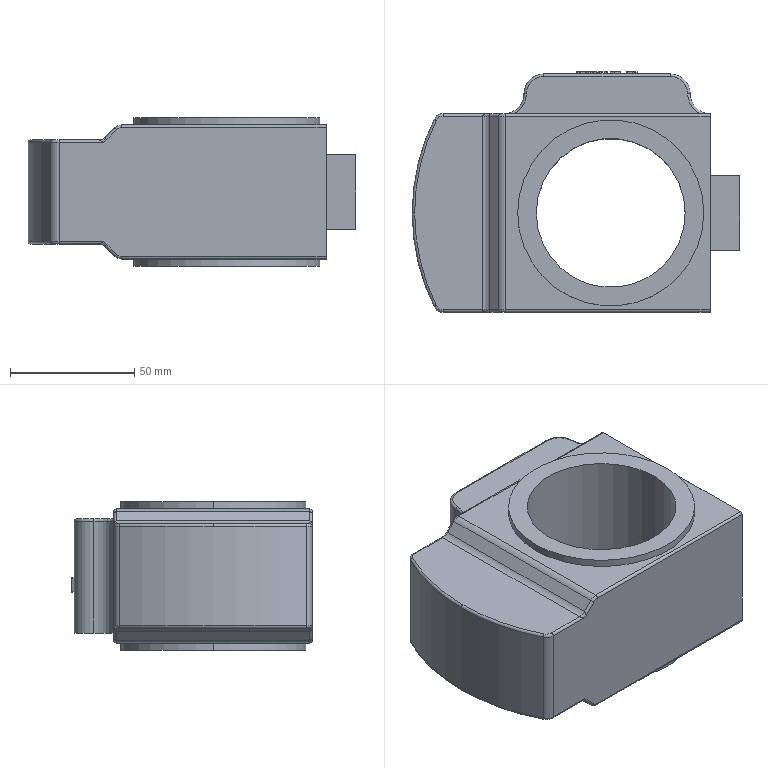Part | SolidWorks | features ICE 6, Fillet 3, Emboss 1, Extrusion 1, MirrorPattern 1 | 1 solid | 143 faces | box 132 x 97 x 60 mm | volume 392584 mm3 | plane 56 | spline 42 | cylinder 30 | torus 15 | commonest cylinder face diameters 2 x13 8 x6 16 x4 75 x4 60 x2 170 x1